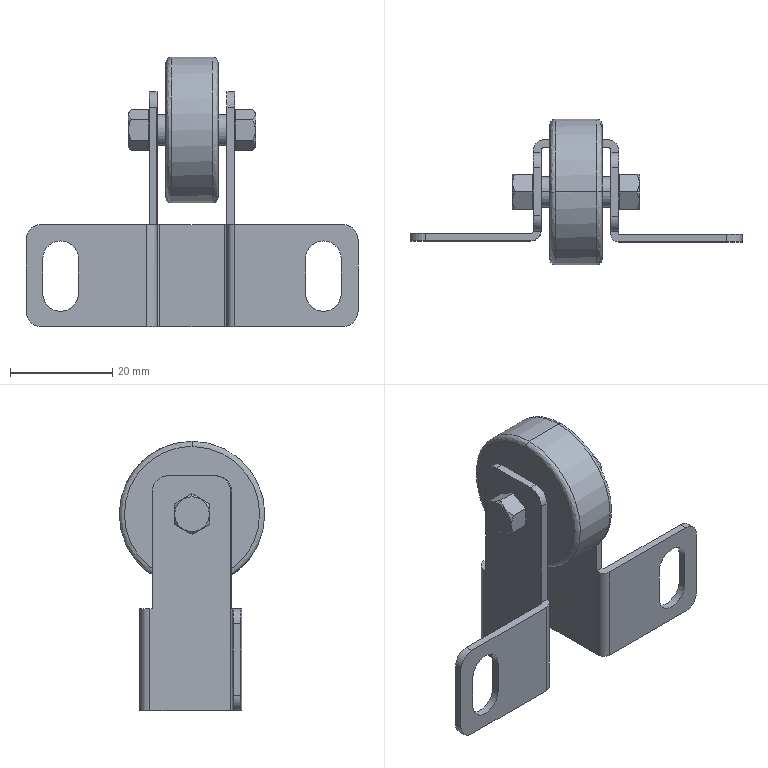Part | SolidWorks | features BaseBody 1 | 1 solid | 83 faces | box 65.06 x 28.5 x 52.75 mm | volume 10830 mm3 | plane 44 | cylinder 31 | cone 4 | spline 4 | commonest cylinder face diameters 6 x16 7 x6 1 x3 4 x3 28.5 x2 3 x1